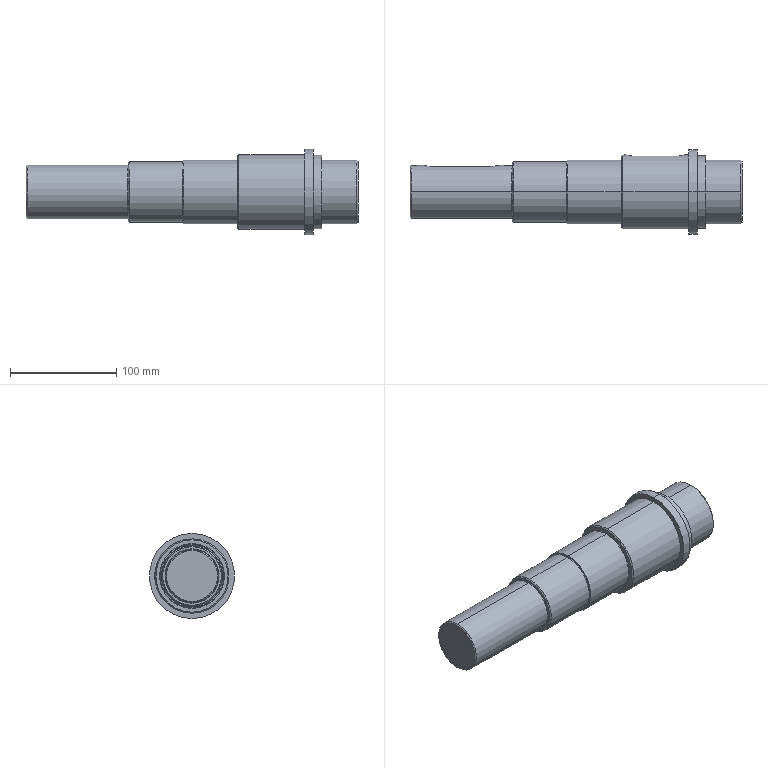Part | SolidWorks | features Chamfer 4, Fillet 2, ICE 2, Revolution 1 | 1 solid | 46 faces | box 312 x 80 x 80 mm | volume 861601 mm3 | cylinder 18 | plane 14 | cone 8 | torus 6 | commonest cylinder face diameters 60 x4 14 x2 20 x2 50 x2 57 x2 69 x2
STEP:
#1=CARTESIAN_POINT('',(199.,0.,30.5));
#2=VERTEX_POINT('',#1);
#3=CARTESIAN_POINT('',(199.,0.,-30.5));
#4=VERTEX_POINT('',#3);
#5=CARTESIAN_POINT('',(199.,0.,0.));
#6=DIRECTION('',(1.,0.,0.));
#7=DIRECTION('',(0.,0.,-1.));
#8=AXIS2_PLACEMENT_3D('',#5,#6,#7);
#9=CIRCLE('',#8,30.5);
#10=EDGE_CURVE('',#2,#4,#9,.T.);
#11=ORIENTED_EDGE('',*,*,#10,.F.);
#12=CARTESIAN_POINT('',(198.5,0.,30.));
#13=VERTEX_POINT('',#12);
#14=CARTESIAN_POINT('',(198.5,0.,30.5));
#15=DIRECTION('',(0.,1.,0.));
#16=DIRECTION('',(0.,0.,1.));
#17=AXIS2_PLACEMENT_3D('',#14,#15,#16);
#18=CIRCLE('',#17,0.5);
#19=EDGE_CURVE('',#2,#13,#18,.T.);
#20=ORIENTED_EDGE('',*,*,#19,.T.);
#21=CARTESIAN_POINT('',(198.5,0.,-30.));
#22=VERTEX_POINT('',#21);
#23=CARTESIAN_POINT('',(198.5,0.,0.));
#24=DIRECTION('',(-1.,0.,0.));
#25=DIRECTION('',(0.,0.,-1.));
#26=AXIS2_PLACEMENT_3D('',#23,#24,#25);
#27=CIRCLE('',#26,30.);
#28=EDGE_CURVE('',#22,#13,#27,.T.);
#29=ORIENTED_EDGE('',*,*,#28,.F.);
#30=CARTESIAN_POINT('',(198.5,0.,-30.5));
#31=DIRECTION('',(0.,-1.,0.));
#32=DIRECTION('',(0.,0.,-1.));
#33=AXIS2_PLACEMENT_3D('',#30,#31,#32);
#34=CIRCLE('',#33,0.5);
#35=EDGE_CURVE('',#4,#22,#34,.T.);
#36=ORIENTED_EDGE('',*,*,#35,.F.);
#37=EDGE_LOOP('',(#11,#20,#29,#36));
#38=FACE_OUTER_BOUND('',#37,.T.);
#39=CARTESIAN_POINT('',(198.5,0.,0.));
#40=DIRECTION('',(1.,0.,0.));
#41=DIRECTION('',(0.,0.,-1.));
#42=AXIS2_PLACEMENT_3D('',#39,#40,#41);
#43=TOROIDAL_SURFACE('',#42,30.5,0.5);
#44=ADVANCED_FACE('',(#38),#43,.F.);
#45=CARTESIAN_POINT('',(96.,0.,27.5));
#46=VERTEX_POINT('',#45);
#47=CARTESIAN_POINT('',(96.,0.,-27.5));
#48=VERTEX_POINT('',#47);
#49=CARTESIAN_POINT('',(96.,0.,0.));
#50=DIRECTION('',(-1.,0.,0.));
#51=DIRECTION('',(0.,0.,-1.));
#52=AXIS2_PLACEMENT_3D('',#49,#50,#51);
#53=CIRCLE('',#52,27.5);
#54=EDGE_CURVE('',#46,#48,#53,.T.);
#55=ORIENTED_EDGE('',*,*,#54,.F.);
#56=CARTESIAN_POINT('',(97.,0.,28.5));
#57=VERTEX_POINT('',#56);
#58=CARTESIAN_POINT('',(96.,0.,27.5));
#59=DIRECTION('',(0.7071,0.,0.7071));
#60=VECTOR('',#59,1000.);
#61=LINE('',#58,#60);
#62=EDGE_CURVE('',#46,#57,#61,.T.);
#63=ORIENTED_EDGE('',*,*,#62,.T.);
#64=CARTESIAN_POINT('',(97.,0.,-28.5));
#65=VERTEX_POINT('',#64);
#66=CARTESIAN_POINT('',(97.,0.,0.));
#67=DIRECTION('',(1.,0.,0.));
#68=DIRECTION('',(0.,0.,-1.));
#69=AXIS2_PLACEMENT_3D('',#66,#67,#68);
#70=CIRCLE('',#69,28.5);
#71=EDGE_CURVE('',#65,#57,#70,.T.);
#72=ORIENTED_EDGE('',*,*,#71,.F.);
#73=CARTESIAN_POINT('',(96.,0.,-27.5));
#74=DIRECTION('',(0.7071,0.,-0.7071));
#75=VECTOR('',#74,1000.);
#76=LINE('',#73,#75);
#77=EDGE_CURVE('',#48,#65,#76,.T.);
#78=ORIENTED_EDGE('',*,*,#77,.F.);
#79=EDGE_LOOP('',(#55,#63,#72,#78));
#80=FACE_OUTER_BOUND('',#79,.T.);
#81=CARTESIAN_POINT('',(96.,0.,0.));
#82=DIRECTION('',(1.,0.,0.));
#83=DIRECTION('',(0.,0.,-1.));
#84=AXIS2_PLACEMENT_3D('',#81,#82,#83);
#85=CONICAL_SURFACE('',#84,27.5,0.7854);
#86=ADVANCED_FACE('',(#80),#85,.T.);
#87=CARTESIAN_POINT('',(199.,0.,34.));
#88=VERTEX_POINT('',#87);
#89=CARTESIAN_POINT('',(199.,0.,-34.));
#90=VERTEX_POINT('',#89);
#91=CARTESIAN_POINT('',(199.,0.,0.));
#92=DIRECTION('',(-1.,0.,0.));
#93=DIRECTION('',(0.,0.,-1.));
#94=AXIS2_PLACEMENT_3D('',#91,#92,#93);
#95=CIRCLE('',#94,34.);
#96=EDGE_CURVE('',#88,#90,#95,.T.);
#97=ORIENTED_EDGE('',*,*,#96,.F.);
#98=CARTESIAN_POINT('',(200.,0.,35.));
#99=VERTEX_POINT('',#98);
#100=CARTESIAN_POINT('',(199.,0.,34.));
#101=DIRECTION('',(0.7071,0.,0.7071));
#102=VECTOR('',#101,1000.);
#103=LINE('',#100,#102);
#104=EDGE_CURVE('',#88,#99,#103,.T.);
#105=ORIENTED_EDGE('',*,*,#104,.T.);
#106=CARTESIAN_POINT('',(200.,0.,-35.));
#107=VERTEX_POINT('',#106);
#108=CARTESIAN_POINT('',(200.,0.,0.));
#109=DIRECTION('',(1.,0.,0.));
#110=DIRECTION('',(0.,0.,-1.));
#111=AXIS2_PLACEMENT_3D('',#108,#109,#110);
#112=CIRCLE('',#111,35.);
#113=EDGE_CURVE('',#107,#99,#112,.T.);
#114=ORIENTED_EDGE('',*,*,#113,.F.);
#115=CARTESIAN_POINT('',(199.,0.,-34.));
#116=DIRECTION('',(0.7071,0.,-0.7071));
#117=VECTOR('',#116,1000.);
#118=LINE('',#115,#117);
#119=EDGE_CURVE('',#90,#107,#118,.T.);
#120=ORIENTED_EDGE('',*,*,#119,.F.);
#121=EDGE_LOOP('',(#97,#105,#114,#120));
#122=FACE_OUTER_BOUND('',#121,.T.);
#123=CARTESIAN_POINT('',(199.,0.,0.));
#124=DIRECTION('',(1.,0.,0.));
#125=DIRECTION('',(0.,0.,-1.));
#126=AXIS2_PLACEMENT_3D('',#123,#124,#125);
#127=CONICAL_SURFACE('',#126,34.,0.7854);
#128=ADVANCED_FACE('',(#122),#127,.T.);
#129=CARTESIAN_POINT('',(96.,0.,25.5));
#130=VERTEX_POINT('',#129);
#131=CARTESIAN_POINT('',(96.,0.,-25.5));
#132=VERTEX_POINT('',#131);
#133=CARTESIAN_POINT('',(96.,0.,0.));
#134=DIRECTION('',(1.,0.,0.));
#135=DIRECTION('',(0.,0.,-1.));
#136=AXIS2_PLACEMENT_3D('',#133,#134,#135);
#137=CIRCLE('',#136,25.5);
#138=EDGE_CURVE('',#130,#132,#137,.T.);
#139=ORIENTED_EDGE('',*,*,#138,.F.);
#140=CARTESIAN_POINT('',(95.5,0.,25.));
#141=VERTEX_POINT('',#140);
#142=CARTESIAN_POINT('',(95.5,0.,25.5));
#143=DIRECTION('',(0.,1.,0.));
#144=DIRECTION('',(0.,0.,1.));
#145=AXIS2_PLACEMENT_3D('',#142,#143,#144);
#146=CIRCLE('',#145,0.5);
#147=EDGE_CURVE('',#130,#141,#146,.T.);
#148=ORIENTED_EDGE('',*,*,#147,.T.);
#149=CARTESIAN_POINT('',(95.5,0.,-25.));
#150=VERTEX_POINT('',#149);
#151=CARTESIAN_POINT('',(95.5,0.,0.));
#152=DIRECTION('',(-1.,0.,0.));
#153=DIRECTION('',(0.,0.,-1.));
#154=AXIS2_PLACEMENT_3D('',#151,#152,#153);
#155=CIRCLE('',#154,25.);
#156=EDGE_CURVE('',#150,#141,#155,.T.);
#157=ORIENTED_EDGE('',*,*,#156,.F.);
#158=CARTESIAN_POINT('',(95.5,0.,-25.5));
#159=DIRECTION('',(0.,-1.,0.));
#160=DIRECTION('',(0.,0.,-1.));
#161=AXIS2_PLACEMENT_3D('',#158,#159,#160);
#162=CIRCLE('',#161,0.5);
#163=EDGE_CURVE('',#132,#150,#162,.T.);
#164=ORIENTED_EDGE('',*,*,#163,.F.);
#165=EDGE_LOOP('',(#139,#148,#157,#164));
#166=FACE_OUTER_BOUND('',#165,.T.);
#167=CARTESIAN_POINT('',(95.5,0.,0.));
#168=DIRECTION('',(1.,0.,0.));
#169=DIRECTION('',(0.,0.,-1.));
#170=AXIS2_PLACEMENT_3D('',#167,#168,#169);
#171=TOROIDAL_SURFACE('',#170,25.5,0.5);
#172=ADVANCED_FACE('',(#166),#171,.F.);
#173=CARTESIAN_POINT('',(148.,0.,29.));
#174=VERTEX_POINT('',#173);
#175=CARTESIAN_POINT('',(148.,0.,-29.));
#176=VERTEX_POINT('',#175);
#177=CARTESIAN_POINT('',(148.,0.,0.));
#178=DIRECTION('',(1.,0.,0.));
#179=DIRECTION('',(0.,0.,-1.));
#180=AXIS2_PLACEMENT_3D('',#177,#178,#179);
#181=CIRCLE('',#180,29.);
#182=EDGE_CURVE('',#174,#176,#181,.T.);
#183=ORIENTED_EDGE('',*,*,#182,.F.);
#184=CARTESIAN_POINT('',(147.5,0.,28.5));
#185=VERTEX_POINT('',#184);
#186=CARTESIAN_POINT('',(147.5,0.,29.));
#187=DIRECTION('',(0.,1.,0.));
#188=DIRECTION('',(0.,0.,1.));
#189=AXIS2_PLACEMENT_3D('',#186,#187,#188);
#190=CIRCLE('',#189,0.5);
#191=EDGE_CURVE('',#174,#185,#190,.T.);
#192=ORIENTED_EDGE('',*,*,#191,.T.);
#193=CARTESIAN_POINT('',(147.5,0.,-28.5));
#194=VERTEX_POINT('',#193);
#195=CARTESIAN_POINT('',(147.5,0.,0.));
#196=DIRECTION('',(-1.,0.,0.));
#197=DIRECTION('',(0.,0.,-1.));
#198=AXIS2_PLACEMENT_3D('',#195,#196,#197);
#199=CIRCLE('',#198,28.5);
#200=EDGE_CURVE('',#194,#185,#199,.T.);
#201=ORIENTED_EDGE('',*,*,#200,.F.);
#202=CARTESIAN_POINT('',(147.5,0.,-29.));
#203=DIRECTION('',(0.,-1.,0.));
#204=DIRECTION('',(0.,0.,-1.));
#205=AXIS2_PLACEMENT_3D('',#202,#203,#204);
#206=CIRCLE('',#205,0.5);
#207=EDGE_CURVE('',#176,#194,#206,.T.);
#208=ORIENTED_EDGE('',*,*,#207,.F.);
#209=EDGE_LOOP('',(#183,#192,#201,#208));
#210=FACE_OUTER_BOUND('',#209,.T.);
#211=CARTESIAN_POINT('',(147.5,0.,0.));
#212=DIRECTION('',(1.,0.,0.));
#213=DIRECTION('',(0.,0.,-1.));
#214=AXIS2_PLACEMENT_3D('',#211,#212,#213);
#215=TOROIDAL_SURFACE('',#214,29.,0.5);
#216=ADVANCED_FACE('',(#210),#215,.F.);
#217=CARTESIAN_POINT('',(312.,0.,-29.));
#218=VERTEX_POINT('',#217);
#219=CARTESIAN_POINT('',(312.,0.,29.));
#220=VERTEX_POINT('',#219);
#221=CARTESIAN_POINT('',(312.,0.,0.));
#222=DIRECTION('',(1.,0.,0.));
#223=DIRECTION('',(0.,0.,1.));
#224=AXIS2_PLACEMENT_3D('',#221,#222,#223);
#225=CIRCLE('',#224,29.);
#226=EDGE_CURVE('',#218,#220,#225,.T.);
#227=ORIENTED_EDGE('',*,*,#226,.F.);
#228=CARTESIAN_POINT('',(311.,0.,-30.));
#229=VERTEX_POINT('',#228);
#230=CARTESIAN_POINT('',(311.,0.,-30.));
#231=DIRECTION('',(-0.7071,0.,-0.7071));
#232=VECTOR('',#231,1000.);
#233=LINE('',#230,#232);
#234=EDGE_CURVE('',#218,#229,#233,.T.);
#235=ORIENTED_EDGE('',*,*,#234,.T.);
#236=CARTESIAN_POINT('',(311.,0.,30.));
#237=VERTEX_POINT('',#236);
#238=CARTESIAN_POINT('',(311.,0.,0.));
#239=DIRECTION('',(-1.,0.,0.));
#240=DIRECTION('',(0.,0.,1.));
#241=AXIS2_PLACEMENT_3D('',#238,#239,#240);
#242=CIRCLE('',#241,30.);
#243=EDGE_CURVE('',#237,#229,#242,.T.);
#244=ORIENTED_EDGE('',*,*,#243,.F.);
#245=CARTESIAN_POINT('',(311.,0.,30.));
#246=DIRECTION('',(-0.7071,0.,0.7071));
#247=VECTOR('',#246,1000.);
#248=LINE('',#245,#247);
#249=EDGE_CURVE('',#220,#237,#248,.T.);
#250=ORIENTED_EDGE('',*,*,#249,.F.);
#251=EDGE_LOOP('',(#227,#235,#244,#250));
#252=FACE_OUTER_BOUND('',#251,.T.);
#253=CARTESIAN_POINT('',(311.,0.,0.));
#254=DIRECTION('',(-1.,0.,0.));
#255=DIRECTION('',(0.,0.,1.));
#256=AXIS2_PLACEMENT_3D('',#253,#254,#255);
#257=CONICAL_SURFACE('',#256,30.,0.7854);
#258=ADVANCED_FACE('',(#252),#257,.T.);
#259=CARTESIAN_POINT('',(0.,0.,24.));
#260=VERTEX_POINT('',#259);
#261=CARTESIAN_POINT('',(0.,0.,-24.));
#262=VERTEX_POINT('',#261);
#263=CARTESIAN_POINT('',(0.,0.,0.));
#264=DIRECTION('',(-1.,0.,0.));
#265=DIRECTION('',(0.,0.,-1.));
#266=AXIS2_PLACEMENT_3D('',#263,#264,#265);
#267=CIRCLE('',#266,24.);
#268=EDGE_CURVE('',#260,#262,#267,.T.);
#269=ORIENTED_EDGE('',*,*,#268,.F.);
#270=CARTESIAN_POINT('',(1.,0.,25.));
#271=VERTEX_POINT('',#270);
#272=CARTESIAN_POINT('',(0.,0.,24.));
#273=DIRECTION('',(0.7071,0.,0.7071));
#274=VECTOR('',#273,1000.);
#275=LINE('',#272,#274);
#276=EDGE_CURVE('',#260,#271,#275,.T.);
#277=ORIENTED_EDGE('',*,*,#276,.T.);
#278=CARTESIAN_POINT('',(1.,0.,-25.));
#279=VERTEX_POINT('',#278);
#280=CARTESIAN_POINT('',(1.,0.,0.));
#281=DIRECTION('',(1.,0.,0.));
#282=DIRECTION('',(0.,0.,-1.));
#283=AXIS2_PLACEMENT_3D('',#280,#281,#282);
#284=CIRCLE('',#283,25.);
#285=EDGE_CURVE('',#279,#271,#284,.T.);
#286=ORIENTED_EDGE('',*,*,#285,.F.);
#287=CARTESIAN_POINT('',(0.,0.,-24.));
#288=DIRECTION('',(0.7071,0.,-0.7071));
#289=VECTOR('',#288,1000.);
#290=LINE('',#287,#289);
#291=EDGE_CURVE('',#262,#279,#290,.T.);
#292=ORIENTED_EDGE('',*,*,#291,.F.);
#293=EDGE_LOOP('',(#269,#277,#286,#292));
#294=FACE_OUTER_BOUND('',#293,.T.);
#295=CARTESIAN_POINT('',(0.,0.,0.));
#296=DIRECTION('',(1.,0.,0.));
#297=DIRECTION('',(0.,0.,-1.));
#298=AXIS2_PLACEMENT_3D('',#295,#296,#297);
#299=CONICAL_SURFACE('',#298,24.,0.7854);
#300=ADVANCED_FACE('',(#294),#299,.T.);
#301=ORIENTED_EDGE('',*,*,#243,.T.);
#302=CARTESIAN_POINT('',(278.,0.,-30.));
#303=VERTEX_POINT('',#302);
#304=CARTESIAN_POINT('',(0.,0.,-30.));
#305=DIRECTION('',(-1.,0.,0.));
#306=VECTOR('',#305,1000.);
#307=LINE('',#304,#306);
#308=EDGE_CURVE('',#229,#303,#307,.T.);
#309=ORIENTED_EDGE('',*,*,#308,.T.);
#310=CARTESIAN_POINT('',(278.,0.,30.));
#311=VERTEX_POINT('',#310);
#312=CARTESIAN_POINT('',(278.,0.,0.));
#313=DIRECTION('',(-1.,0.,0.));
#314=DIRECTION('',(0.,0.,1.));
#315=AXIS2_PLACEMENT_3D('',#312,#313,#314);
#316=CIRCLE('',#315,30.);
#317=EDGE_CURVE('',#311,#303,#316,.T.);
#318=ORIENTED_EDGE('',*,*,#317,.F.);
#319=CARTESIAN_POINT('',(0.,0.,30.));
#320=DIRECTION('',(-1.,0.,0.));
#321=VECTOR('',#320,1000.);
#322=LINE('',#319,#321);
#323=EDGE_CURVE('',#237,#311,#322,.T.);
#324=ORIENTED_EDGE('',*,*,#323,.F.);
#325=EDGE_LOOP('',(#301,#309,#318,#324));
#326=FACE_OUTER_BOUND('',#325,.T.);
#327=CARTESIAN_POINT('',(0.,0.,0.));
#328=DIRECTION('',(-1.,0.,0.));
#329=DIRECTION('',(0.,0.,1.));
#330=AXIS2_PLACEMENT_3D('',#327,#328,#329);
#331=CYLINDRICAL_SURFACE('',#330,30.);
#332=ADVANCED_FACE('',(#326),#331,.T.);
#333=CARTESIAN_POINT('',(278.,0.,34.5));
#334=VERTEX_POINT('',#333);
#335=CARTESIAN_POINT('',(278.,0.,-34.5));
#336=VERTEX_POINT('',#335);
#337=CARTESIAN_POINT('',(278.,0.,0.));
#338=DIRECTION('',(-1.,0.,0.));
#339=DIRECTION('',(0.,0.,1.));
#340=AXIS2_PLACEMENT_3D('',#337,#338,#339);
#341=CIRCLE('',#340,34.5);
#342=EDGE_CURVE('',#334,#336,#341,.T.);
#343=ORIENTED_EDGE('',*,*,#342,.T.);
#344=CARTESIAN_POINT('',(270.,0.,-34.5));
#345=VERTEX_POINT('',#344);
#346=CARTESIAN_POINT('',(0.,0.,-34.5));
#347=DIRECTION('',(-1.,0.,0.));
#348=VECTOR('',#347,1000.);
#349=LINE('',#346,#348);
#350=EDGE_CURVE('',#336,#345,#349,.T.);
#351=ORIENTED_EDGE('',*,*,#350,.T.);
#352=CARTESIAN_POINT('',(270.,0.,34.5));
#353=VERTEX_POINT('',#352);
#354=CARTESIAN_POINT('',(270.,0.,0.));
#355=DIRECTION('',(-1.,0.,0.));
#356=DIRECTION('',(0.,0.,1.));
#357=AXIS2_PLACEMENT_3D('',#354,#355,#356);
#358=CIRCLE('',#357,34.5);
#359=EDGE_CURVE('',#353,#345,#358,.T.);
#360=ORIENTED_EDGE('',*,*,#359,.F.);
#361=CARTESIAN_POINT('',(0.,0.,34.5));
#362=DIRECTION('',(-1.,0.,0.));
#363=VECTOR('',#362,1000.);
#364=LINE('',#361,#363);
#365=EDGE_CURVE('',#334,#353,#364,.T.);
#366=ORIENTED_EDGE('',*,*,#365,.F.);
#367=EDGE_LOOP('',(#343,#351,#360,#366));
#368=FACE_OUTER_BOUND('',#367,.T.);
#369=CARTESIAN_POINT('',(0.,0.,0.));
#370=DIRECTION('',(-1.,0.,0.));
#371=DIRECTION('',(0.,0.,1.));
#372=AXIS2_PLACEMENT_3D('',#369,#370,#371);
#373=CYLINDRICAL_SURFACE('',#372,34.5);
#374=ADVANCED_FACE('',(#368),#373,.T.);
#375=CARTESIAN_POINT('',(270.,0.,40.));
#376=VERTEX_POINT('',#375);
#377=CARTESIAN_POINT('',(270.,0.,-40.));
#378=VERTEX_POINT('',#377);
#379=CARTESIAN_POINT('',(270.,0.,0.));
#380=DIRECTION('',(-1.,0.,0.));
#381=DIRECTION('',(0.,0.,1.));
#382=AXIS2_PLACEMENT_3D('',#379,#380,#381);
#383=CIRCLE('',#382,40.);
#384=EDGE_CURVE('',#376,#378,#383,.T.);
#385=ORIENTED_EDGE('',*,*,#384,.T.);
#386=CARTESIAN_POINT('',(262.,0.,-40.));
#387=VERTEX_POINT('',#386);
#388=CARTESIAN_POINT('',(0.,0.,-40.));
#389=DIRECTION('',(-1.,0.,0.));
#390=VECTOR('',#389,1000.);
#391=LINE('',#388,#390);
#392=EDGE_CURVE('',#378,#387,#391,.T.);
#393=ORIENTED_EDGE('',*,*,#392,.T.);
#394=CARTESIAN_POINT('',(262.,0.,40.));
#395=VERTEX_POINT('',#394);
#396=CARTESIAN_POINT('',(262.,0.,0.));
#397=DIRECTION('',(-1.,0.,0.));
#398=DIRECTION('',(0.,0.,1.));
#399=AXIS2_PLACEMENT_3D('',#396,#397,#398);
#400=CIRCLE('',#399,40.);
#401=EDGE_CURVE('',#395,#387,#400,.T.);
#402=ORIENTED_EDGE('',*,*,#401,.F.);
#403=CARTESIAN_POINT('',(0.,0.,40.));
#404=DIRECTION('',(-1.,0.,0.));
#405=VECTOR('',#404,1000.);
#406=LINE('',#403,#405);
#407=EDGE_CURVE('',#376,#395,#406,.T.);
#408=ORIENTED_EDGE('',*,*,#407,.F.);
#409=EDGE_LOOP('',(#385,#393,#402,#408));
#410=FACE_OUTER_BOUND('',#409,.T.);
#411=CARTESIAN_POINT('',(0.,0.,0.));
#412=DIRECTION('',(-1.,0.,0.));
#413=DIRECTION('',(0.,0.,1.));
#414=AXIS2_PLACEMENT_3D('',#411,#412,#413);
#415=CYLINDRICAL_SURFACE('',#414,40.);
#416=ADVANCED_FACE('',(#410),#415,.T.);
#417=CARTESIAN_POINT('',(198.5,0.,0.));
#418=DIRECTION('',(-1.,0.,0.));
#419=DIRECTION('',(0.,0.,-1.));
#420=AXIS2_PLACEMENT_3D('',#417,#418,#419);
#421=CIRCLE('',#420,30.);
#422=EDGE_CURVE('',#13,#22,#421,.T.);
#423=ORIENTED_EDGE('',*,*,#422,.T.);
#424=CARTESIAN_POINT('',(148.,0.,-30.));
#425=VERTEX_POINT('',#424);
#426=CARTESIAN_POINT('',(0.,0.,-30.));
#427=DIRECTION('',(-1.,0.,0.));
#428=VECTOR('',#427,1000.);
#429=LINE('',#426,#428);
#430=EDGE_CURVE('',#22,#425,#429,.T.);
#431=ORIENTED_EDGE('',*,*,#430,.T.);
#432=CARTESIAN_POINT('',(148.,0.,30.));
#433=VERTEX_POINT('',#432);
#434=CARTESIAN_POINT('',(148.,0.,0.));
#435=DIRECTION('',(-1.,0.,0.));
#436=DIRECTION('',(0.,0.,1.));
#437=AXIS2_PLACEMENT_3D('',#434,#435,#436);
#438=CIRCLE('',#437,30.);
#439=EDGE_CURVE('',#433,#425,#438,.T.);
#440=ORIENTED_EDGE('',*,*,#439,.F.);
#441=CARTESIAN_POINT('',(0.,0.,30.));
#442=DIRECTION('',(-1.,0.,0.));
#443=VECTOR('',#442,1000.);
#444=LINE('',#441,#443);
#445=EDGE_CURVE('',#13,#433,#444,.T.);
#446=ORIENTED_EDGE('',*,*,#445,.F.);
#447=EDGE_LOOP('',(#423,#431,#440,#446));
#448=FACE_OUTER_BOUND('',#447,.T.);
#449=CARTESIAN_POINT('',(0.,0.,0.));
#450=DIRECTION('',(-1.,0.,0.));
#451=DIRECTION('',(0.,0.,1.));
#452=AXIS2_PLACEMENT_3D('',#449,#450,#451);
#453=CYLINDRICAL_SURFACE('',#452,30.);
#454=ADVANCED_FACE('',(#448),#453,.T.);
#455=CARTESIAN_POINT('',(147.5,0.,0.));
#456=DIRECTION('',(-1.,0.,0.));
#457=DIRECTION('',(0.,0.,-1.));
#458=AXIS2_PLACEMENT_3D('',#455,#456,#457);
#459=CIRCLE('',#458,28.5);
#460=EDGE_CURVE('',#185,#194,#459,.T.);
#461=ORIENTED_EDGE('',*,*,#460,.T.);
#462=CARTESIAN_POINT('',(0.,0.,-28.5));
#463=DIRECTION('',(-1.,0.,0.));
#464=VECTOR('',#463,1000.);
#465=LINE('',#462,#464);
#466=EDGE_CURVE('',#194,#65,#465,.T.);
#467=ORIENTED_EDGE('',*,*,#466,.T.);
#468=ORIENTED_EDGE('',*,*,#71,.T.);
#469=CARTESIAN_POINT('',(0.,0.,28.5));
#470=DIRECTION('',(-1.,0.,0.));
#471=VECTOR('',#470,1000.);
#472=LINE('',#469,#471);
#473=EDGE_CURVE('',#185,#57,#472,.T.);
#474=ORIENTED_EDGE('',*,*,#473,.F.);
#475=EDGE_LOOP('',(#461,#467,#468,#474));
#476=FACE_OUTER_BOUND('',#475,.T.);
#477=CARTESIAN_POINT('',(0.,0.,0.));
#478=DIRECTION('',(-1.,0.,0.));
#479=DIRECTION('',(0.,0.,1.));
#480=AXIS2_PLACEMENT_3D('',#477,#478,#479);
#481=CYLINDRICAL_SURFACE('',#480,28.5);
#482=ADVANCED_FACE('',(#476),#481,.T.);
#483=CARTESIAN_POINT('',(20.,24.,-7.));
#484=VERTEX_POINT('',#483);
#485=CARTESIAN_POINT('',(20.,24.,7.));
#486=VERTEX_POINT('',#485);
#487=CARTESIAN_POINT('',(20.,24.,-7.));
#488=CARTESIAN_POINT('',(19.535,24.,-7.));
#489=CARTESIAN_POINT('',(19.079,24.014,-6.954));
#490=CARTESIAN_POINT('',(18.405,24.052,-6.82));
#491=CARTESIAN_POINT('',(18.183,24.068,-6.764));
#492=CARTESIAN_POINT('',(17.742,24.105,-6.63));
#493=CARTESIAN_POINT('',(17.524,24.126,-6.551));
#494=CARTESIAN_POINT('',(16.889,24.197,-6.287));
#495=CARTESIAN_POINT('',(16.488,24.253,-6.072));
#496=CARTESIAN_POINT('',(15.919,24.344,-5.692));
#497=CARTESIAN_POINT('',(15.733,24.376,-5.554));
#498=CARTESIAN_POINT('',(15.38,24.44,-5.263));
#499=CARTESIAN_POINT('',(15.211,24.473,-5.11));
#500=CARTESIAN_POINT('',(14.729,24.57,-4.629));
#501=CARTESIAN_POINT('',(14.44,24.634,-4.278));
#502=CARTESIAN_POINT('',(13.929,24.755,-3.514));
#503=CARTESIAN_POINT('',(13.713,24.809,-3.11));
#504=CARTESIAN_POINT('',(13.45,24.878,-2.48));
#505=CARTESIAN_POINT('',(13.373,24.898,-2.265));
#506=CARTESIAN_POINT('',(13.238,24.934,-1.825));
#507=CARTESIAN_POINT('',(13.181,24.95,-1.6));
#508=CARTESIAN_POINT('',(13.046,24.987,-0.9213));
#509=CARTESIAN_POINT('',(13.,25.,-0.4657));
#510=CARTESIAN_POINT('',(13.,25.,0.4524));
#511=CARTESIAN_POINT('',(13.045,24.987,0.9188));
#512=CARTESIAN_POINT('',(13.225,24.938,1.818));
#513=CARTESIAN_POINT('',(13.358,24.902,2.256));
#514=CARTESIAN_POINT('',(13.622,24.833,2.894));
#515=CARTESIAN_POINT('',(13.721,24.808,3.103));
#516=CARTESIAN_POINT('',(13.937,24.754,3.506));
#517=CARTESIAN_POINT('',(14.054,24.725,3.701));
#518=CARTESIAN_POINT('',(14.307,24.666,4.079));
#519=CARTESIAN_POINT('',(14.442,24.635,4.262));
#520=CARTESIAN_POINT('',(14.732,24.571,4.615));
#521=CARTESIAN_POINT('',(14.887,24.538,4.786));
#522=CARTESIAN_POINT('',(15.372,24.44,5.272));
#523=CARTESIAN_POINT('',(15.722,24.375,5.56));
#524=CARTESIAN_POINT('',(16.478,24.254,6.067));
#525=CARTESIAN_POINT('',(16.888,24.197,6.287));
#526=CARTESIAN_POINT('',(17.731,24.103,6.638));
#527=CARTESIAN_POINT('',(18.168,24.066,6.772));
#528=CARTESIAN_POINT('',(18.844,24.027,6.908));
#529=CARTESIAN_POINT('',(19.075,24.017,6.942));
#530=CARTESIAN_POINT('',(19.536,24.003,6.988));
#531=CARTESIAN_POINT('',(19.768,24.,7.));
#532=CARTESIAN_POINT('',(20.,24.,7.));
#533=B_SPLINE_CURVE_WITH_KNOTS('',3,(#487,#488,#489,#490,#491,#492,#493,#494,#495,#496,#497,#498,#499,#500,#501,#502,#503,#504,#505,#506,#507,#508,#509,#510,#511,#512,#513,#514,#515,#516,#517,#518,#519,#520,#521,#522,#523,#524,#525,#526,#527,#528,#529,#530,#531,#532),.UNSPECIFIED.,.F.,.F.,(4,2,2,2,2,2,2,2,2,2,2,2,2,2,2,2,2,2,2,2,2,2,4),(0.,0.001374,0.002061,0.002749,0.004123,0.00481,0.005497,0.006871,0.008246,0.008933,0.00962,0.01099,0.01237,0.01374,0.01443,0.01512,0.0158,0.01649,0.01787,0.01924,0.02061,0.0213,0.02199),.UNSPECIFIED.);
#534=EDGE_CURVE('',#484,#486,#533,.T.);
#535=ORIENTED_EDGE('',*,*,#534,.F.);
#536=CARTESIAN_POINT('',(76.,24.,-7.));
#537=VERTEX_POINT('',#536);
#538=CARTESIAN_POINT('',(0.,24.,-7.));
#539=DIRECTION('',(-1.,0.,0.));
#540=VECTOR('',#539,1000.);
#541=LINE('',#538,#540);
#542=EDGE_CURVE('',#537,#484,#541,.T.);
#543=ORIENTED_EDGE('',*,*,#542,.F.);
#544=CARTESIAN_POINT('',(76.,24.,7.));
#545=VERTEX_POINT('',#544);
#546=CARTESIAN_POINT('',(76.,24.,7.));
#547=CARTESIAN_POINT('',(76.465,24.,7.));
#548=CARTESIAN_POINT('',(76.921,24.014,6.954));
#549=CARTESIAN_POINT('',(77.595,24.052,6.82));
#550=CARTESIAN_POINT('',(77.817,24.068,6.764));
#551=CARTESIAN_POINT('',(78.258,24.105,6.63));
#552=CARTESIAN_POINT('',(78.476,24.126,6.551));
#553=CARTESIAN_POINT('',(79.111,24.197,6.287));
#554=CARTESIAN_POINT('',(79.512,24.253,6.072));
#555=CARTESIAN_POINT('',(80.081,24.344,5.692));
#556=CARTESIAN_POINT('',(80.267,24.376,5.554));
#557=CARTESIAN_POINT('',(80.62,24.44,5.263));
#558=CARTESIAN_POINT('',(80.789,24.473,5.11));
#559=CARTESIAN_POINT('',(81.271,24.57,4.629));
#560=CARTESIAN_POINT('',(81.56,24.634,4.278));
#561=CARTESIAN_POINT('',(82.071,24.755,3.514));
#562=CARTESIAN_POINT('',(82.287,24.809,3.11));
#563=CARTESIAN_POINT('',(82.55,24.878,2.48));
#564=CARTESIAN_POINT('',(82.627,24.898,2.265));
#565=CARTESIAN_POINT('',(82.762,24.934,1.825));
#566=CARTESIAN_POINT('',(82.819,24.95,1.6));
#567=CARTESIAN_POINT('',(82.954,24.987,0.9213));
#568=CARTESIAN_POINT('',(83.,25.,0.4657));
#569=CARTESIAN_POINT('',(83.,25.,-0.4524));
#570=CARTESIAN_POINT('',(82.955,24.987,-0.9188));
#571=CARTESIAN_POINT('',(82.775,24.938,-1.818));
#572=CARTESIAN_POINT('',(82.642,24.902,-2.256));
#573=CARTESIAN_POINT('',(82.378,24.833,-2.894));
#574=CARTESIAN_POINT('',(82.279,24.808,-3.103));
#575=CARTESIAN_POINT('',(82.063,24.754,-3.506));
#576=CARTESIAN_POINT('',(81.946,24.725,-3.701));
#577=CARTESIAN_POINT('',(81.693,24.666,-4.079));
#578=CARTESIAN_POINT('',(81.558,24.635,-4.262));
#579=CARTESIAN_POINT('',(81.268,24.571,-4.615));
#580=CARTESIAN_POINT('',(81.113,24.538,-4.786));
#581=CARTESIAN_POINT('',(80.628,24.44,-5.272));
#582=CARTESIAN_POINT('',(80.278,24.375,-5.56));
#583=CARTESIAN_POINT('',(79.522,24.254,-6.067));
#584=CARTESIAN_POINT('',(79.112,24.197,-6.287));
#585=CARTESIAN_POINT('',(78.269,24.103,-6.638));
#586=CARTESIAN_POINT('',(77.832,24.066,-6.772));
#587=CARTESIAN_POINT('',(77.156,24.027,-6.908));
#588=CARTESIAN_POINT('',(76.925,24.017,-6.942));
#589=CARTESIAN_POINT('',(76.464,24.003,-6.988));
#590=CARTESIAN_POINT('',(76.232,24.,-7.));
#591=CARTESIAN_POINT('',(76.,24.,-7.));
#592=B_SPLINE_CURVE_WITH_KNOTS('',3,(#546,#547,#548,#549,#550,#551,#552,#553,#554,#555,#556,#557,#558,#559,#560,#561,#562,#563,#564,#565,#566,#567,#568,#569,#570,#571,#572,#573,#574,#575,#576,#577,#578,#579,#580,#581,#582,#583,#584,#585,#586,#587,#588,#589,#590,#591),.UNSPECIFIED.,.F.,.F.,(4,2,2,2,2,2,2,2,2,2,2,2,2,2,2,2,2,2,2,2,2,2,4),(0.,0.001374,0.002061,0.002749,0.004123,0.00481,0.005497,0.006871,0.008246,0.008933,0.00962,0.01099,0.01237,0.01374,0.01443,0.01512,0.0158,0.01649,0.01787,0.01924,0.02061,0.0213,0.02199),.UNSPECIFIED.);
#593=EDGE_CURVE('',#545,#537,#592,.T.);
#594=ORIENTED_EDGE('',*,*,#593,.F.);
#595=CARTESIAN_POINT('',(0.,24.,7.));
#596=DIRECTION('',(1.,0.,0.));
#597=VECTOR('',#596,1000.);
#598=LINE('',#595,#597);
#599=EDGE_CURVE('',#486,#545,#598,.T.);
#600=ORIENTED_EDGE('',*,*,#599,.F.);
#601=EDGE_LOOP('',(#535,#543,#594,#600));
#602=FACE_BOUND('',#601,.T.);
#603=CARTESIAN_POINT('',(95.5,0.,0.));
#604=DIRECTION('',(-1.,0.,0.));
#605=DIRECTION('',(0.,0.,-1.));
#606=AXIS2_PLACEMENT_3D('',#603,#604,#605);
#607=CIRCLE('',#606,25.);
#608=EDGE_CURVE('',#141,#150,#607,.T.);
#609=ORIENTED_EDGE('',*,*,#608,.T.);
#610=CARTESIAN_POINT('',(0.,0.,-25.));
#611=DIRECTION('',(-1.,0.,0.));
#612=VECTOR('',#611,1000.);
#613=LINE('',#610,#612);
#614=EDGE_CURVE('',#150,#279,#613,.T.);
#615=ORIENTED_EDGE('',*,*,#614,.T.);
#616=ORIENTED_EDGE('',*,*,#285,.T.);
#617=CARTESIAN_POINT('',(0.,0.,25.));
#618=DIRECTION('',(-1.,0.,0.));
#619=VECTOR('',#618,1000.);
#620=LINE('',#617,#619);
#621=EDGE_CURVE('',#141,#271,#620,.T.);
#622=ORIENTED_EDGE('',*,*,#621,.F.);
#623=EDGE_LOOP('',(#609,#615,#616,#622));
#624=FACE_OUTER_BOUND('',#623,.T.);
#625=CARTESIAN_POINT('',(0.,0.,0.));
#626=DIRECTION('',(-1.,0.,0.));
#627=DIRECTION('',(0.,0.,1.));
#628=AXIS2_PLACEMENT_3D('',#625,#626,#627);
#629=CYLINDRICAL_SURFACE('',#628,25.);
#630=ADVANCED_FACE('',(#602,#624),#629,.T.);
#631=CARTESIAN_POINT('',(212.5,33.541,-10.));
#632=VERTEX_POINT('',#631);
#633=CARTESIAN_POINT('',(212.5,33.541,10.));
#634=VERTEX_POINT('',#633);
#635=CARTESIAN_POINT('',(212.5,33.541,-10.));
#636=CARTESIAN_POINT('',(211.836,33.541,-10.));
#637=CARTESIAN_POINT('',(211.183,33.561,-9.934));
#638=CARTESIAN_POINT('',(210.222,33.617,-9.742));
#639=CARTESIAN_POINT('',(209.904,33.64,-9.663));
#640=CARTESIAN_POINT('',(209.274,33.694,-9.471));
#641=CARTESIAN_POINT('',(208.962,33.726,-9.359));
#642=CARTESIAN_POINT('',(208.055,33.829,-8.982));
#643=CARTESIAN_POINT('',(207.482,33.91,-8.675));
#644=CARTESIAN_POINT('',(206.669,34.043,-8.131));
#645=CARTESIAN_POINT('',(206.405,34.089,-7.934));
#646=CARTESIAN_POINT('',(205.899,34.183,-7.519));
#647=CARTESIAN_POINT('',(205.659,34.231,-7.301));
#648=CARTESIAN_POINT('',(204.971,34.373,-6.613));
#649=CARTESIAN_POINT('',(204.558,34.467,-6.112));
#650=CARTESIAN_POINT('',(203.827,34.642,-5.02));
#651=CARTESIAN_POINT('',(203.518,34.722,-4.444));
#652=CARTESIAN_POINT('',(203.143,34.822,-3.543));
#653=CARTESIAN_POINT('',(203.032,34.852,-3.236));
#654=CARTESIAN_POINT('',(202.841,34.904,-2.608));
#655=CARTESIAN_POINT('',(202.759,34.927,-2.286));
#656=CARTESIAN_POINT('',(202.565,34.981,-1.317));
#657=CARTESIAN_POINT('',(202.501,35.,-0.6655));
#658=CARTESIAN_POINT('',(202.499,35.,0.6464));
#659=CARTESIAN_POINT('',(202.565,34.981,1.313));
#660=CARTESIAN_POINT('',(202.821,34.909,2.598));
#661=CARTESIAN_POINT('',(203.011,34.857,3.223));
#662=CARTESIAN_POINT('',(203.389,34.756,4.135));
#663=CARTESIAN_POINT('',(203.531,34.719,4.433));
#664=CARTESIAN_POINT('',(203.839,34.641,5.009));
#665=CARTESIAN_POINT('',(204.006,34.599,5.288));
#666=CARTESIAN_POINT('',(204.367,34.512,5.828));
#667=CARTESIAN_POINT('',(204.561,34.467,6.089));
#668=CARTESIAN_POINT('',(204.974,34.374,6.593));
#669=CARTESIAN_POINT('',(205.196,34.326,6.838));
#670=CARTESIAN_POINT('',(205.888,34.183,7.531));
#671=CARTESIAN_POINT('',(206.389,34.089,7.942));
#672=CARTESIAN_POINT('',(207.469,33.912,8.666));
#673=CARTESIAN_POINT('',(208.054,33.829,8.981));
#674=CARTESIAN_POINT('',(209.259,33.692,9.483));
#675=CARTESIAN_POINT('',(209.882,33.637,9.674));
#676=CARTESIAN_POINT('',(210.849,33.58,9.868));
#677=CARTESIAN_POINT('',(211.178,33.565,9.918));
#678=CARTESIAN_POINT('',(211.837,33.546,9.983));
#679=CARTESIAN_POINT('',(212.168,33.541,10.));
#680=CARTESIAN_POINT('',(212.5,33.541,10.));
#681=B_SPLINE_CURVE_WITH_KNOTS('',3,(#635,#636,#637,#638,#639,#640,#641,#642,#643,#644,#645,#646,#647,#648,#649,#650,#651,#652,#653,#654,#655,#656,#657,#658,#659,#660,#661,#662,#663,#664,#665,#666,#667,#668,#669,#670,#671,#672,#673,#674,#675,#676,#677,#678,#679,#680),.UNSPECIFIED.,.F.,.F.,(4,2,2,2,2,2,2,2,2,2,2,2,2,2,2,2,2,2,2,2,2,2,4),(0.,0.001964,0.002945,0.003927,0.005891,0.006873,0.007855,0.009818,0.01178,0.01276,0.01375,0.01571,0.01767,0.01964,0.02062,0.0216,0.02258,0.02356,0.02553,0.02749,0.02945,0.03044,0.03142),.UNSPECIFIED.);
#682=EDGE_CURVE('',#632,#634,#681,.T.);
#683=ORIENTED_EDGE('',*,*,#682,.F.);
#684=CARTESIAN_POINT('',(248.5,33.541,-10.));
#685=VERTEX_POINT('',#684);
#686=CARTESIAN_POINT('',(0.,33.541,-10.));
#687=DIRECTION('',(-1.,0.,0.));
#688=VECTOR('',#687,1000.);
#689=LINE('',#686,#688);
#690=EDGE_CURVE('',#685,#632,#689,.T.);
#691=ORIENTED_EDGE('',*,*,#690,.F.);
#692=CARTESIAN_POINT('',(248.5,33.541,10.));
#693=VERTEX_POINT('',#692);
#694=CARTESIAN_POINT('',(248.5,33.541,10.));
#695=CARTESIAN_POINT('',(249.164,33.541,10.));
#696=CARTESIAN_POINT('',(249.817,33.561,9.934));
#697=CARTESIAN_POINT('',(250.778,33.617,9.742));
#698=CARTESIAN_POINT('',(251.096,33.64,9.663));
#699=CARTESIAN_POINT('',(251.726,33.694,9.471));
#700=CARTESIAN_POINT('',(252.038,33.726,9.359));
#701=CARTESIAN_POINT('',(252.945,33.829,8.982));
#702=CARTESIAN_POINT('',(253.518,33.91,8.675));
#703=CARTESIAN_POINT('',(254.331,34.043,8.131));
#704=CARTESIAN_POINT('',(254.595,34.089,7.934));
#705=CARTESIAN_POINT('',(255.101,34.183,7.519));
#706=CARTESIAN_POINT('',(255.341,34.231,7.301));
#707=CARTESIAN_POINT('',(256.029,34.373,6.613));
#708=CARTESIAN_POINT('',(256.442,34.467,6.112));
#709=CARTESIAN_POINT('',(257.173,34.642,5.02));
#710=CARTESIAN_POINT('',(257.482,34.722,4.444));
#711=CARTESIAN_POINT('',(257.857,34.822,3.543));
#712=CARTESIAN_POINT('',(257.968,34.852,3.236));
#713=CARTESIAN_POINT('',(258.159,34.904,2.608));
#714=CARTESIAN_POINT('',(258.241,34.927,2.286));
#715=CARTESIAN_POINT('',(258.435,34.981,1.317));
#716=CARTESIAN_POINT('',(258.499,35.,0.6655));
#717=CARTESIAN_POINT('',(258.501,35.,-0.6464));
#718=CARTESIAN_POINT('',(258.435,34.981,-1.313));
#719=CARTESIAN_POINT('',(258.179,34.909,-2.598));
#720=CARTESIAN_POINT('',(257.989,34.857,-3.223));
#721=CARTESIAN_POINT('',(257.611,34.756,-4.135));
#722=CARTESIAN_POINT('',(257.469,34.719,-4.433));
#723=CARTESIAN_POINT('',(257.161,34.641,-5.009));
#724=CARTESIAN_POINT('',(256.994,34.599,-5.288));
#725=CARTESIAN_POINT('',(256.633,34.512,-5.828));
#726=CARTESIAN_POINT('',(256.439,34.467,-6.089));
#727=CARTESIAN_POINT('',(256.026,34.374,-6.593));
#728=CARTESIAN_POINT('',(255.804,34.326,-6.838));
#729=CARTESIAN_POINT('',(255.112,34.183,-7.531));
#730=CARTESIAN_POINT('',(254.611,34.089,-7.942));
#731=CARTESIAN_POINT('',(253.531,33.912,-8.666));
#732=CARTESIAN_POINT('',(252.946,33.829,-8.981));
#733=CARTESIAN_POINT('',(251.741,33.692,-9.483));
#734=CARTESIAN_POINT('',(251.118,33.637,-9.674));
#735=CARTESIAN_POINT('',(250.151,33.58,-9.868));
#736=CARTESIAN_POINT('',(249.822,33.565,-9.918));
#737=CARTESIAN_POINT('',(249.163,33.546,-9.983));
#738=CARTESIAN_POINT('',(248.832,33.541,-10.));
#739=CARTESIAN_POINT('',(248.5,33.541,-10.));
#740=B_SPLINE_CURVE_WITH_KNOTS('',3,(#694,#695,#696,#697,#698,#699,#700,#701,#702,#703,#704,#705,#706,#707,#708,#709,#710,#711,#712,#713,#714,#715,#716,#717,#718,#719,#720,#721,#722,#723,#724,#725,#726,#727,#728,#729,#730,#731,#732,#733,#734,#735,#736,#737,#738,#739),.UNSPECIFIED.,.F.,.F.,(4,2,2,2,2,2,2,2,2,2,2,2,2,2,2,2,2,2,2,2,2,2,4),(0.,0.001964,0.002945,0.003927,0.005891,0.006873,0.007855,0.009818,0.01178,0.01276,0.01375,0.01571,0.01767,0.01964,0.02062,0.0216,0.02258,0.02356,0.02553,0.02749,0.02945,0.03044,0.03142),.UNSPECIFIED.);
#741=EDGE_CURVE('',#693,#685,#740,.T.);
#742=ORIENTED_EDGE('',*,*,#741,.F.);
#743=CARTESIAN_POINT('',(0.,33.541,10.));
#744=DIRECTION('',(1.,0.,0.));
#745=VECTOR('',#744,1000.);
#746=LINE('',#743,#745);
#747=EDGE_CURVE('',#634,#693,#746,.T.);
#748=ORIENTED_EDGE('',*,*,#747,.F.);
#749=EDGE_LOOP('',(#683,#691,#742,#748));
#750=FACE_BOUND('',#749,.T.);
#751=CARTESIAN_POINT('',(262.,0.,35.));
#752=VERTEX_POINT('',#751);
#753=CARTESIAN_POINT('',(262.,0.,-35.));
#754=VERTEX_POINT('',#753);
#755=CARTESIAN_POINT('',(262.,0.,0.));
#756=DIRECTION('',(-1.,0.,0.));
#757=DIRECTION('',(0.,0.,1.));
#758=AXIS2_PLACEMENT_3D('',#755,#756,#757);
#759=CIRCLE('',#758,35.);
#760=EDGE_CURVE('',#752,#754,#759,.T.);
#761=ORIENTED_EDGE('',*,*,#760,.T.);
#762=CARTESIAN_POINT('',(0.,0.,-35.));
#763=DIRECTION('',(-1.,0.,0.));
#764=VECTOR('',#763,1000.);
#765=LINE('',#762,#764);
#766=EDGE_CURVE('',#754,#107,#765,.T.);
#767=ORIENTED_EDGE('',*,*,#766,.T.);
#768=ORIENTED_EDGE('',*,*,#113,.T.);
#769=CARTESIAN_POINT('',(0.,0.,35.));
#770=DIRECTION('',(-1.,0.,0.));
#771=VECTOR('',#770,1000.);
#772=LINE('',#769,#771);
#773=EDGE_CURVE('',#752,#99,#772,.T.);
#774=ORIENTED_EDGE('',*,*,#773,.F.);
#775=EDGE_LOOP('',(#761,#767,#768,#774));
#776=FACE_OUTER_BOUND('',#775,.T.);
#777=CARTESIAN_POINT('',(0.,0.,0.));
#778=DIRECTION('',(-1.,0.,0.));
#779=DIRECTION('',(0.,0.,1.));
#780=AXIS2_PLACEMENT_3D('',#777,#778,#779);
#781=CYLINDRICAL_SURFACE('',#780,35.);
#782=ADVANCED_FACE('',(#750,#776),#781,.T.);
#783=ORIENTED_EDGE('',*,*,#766,.F.);
#784=CARTESIAN_POINT('',(262.,0.,0.));
#785=DIRECTION('',(-1.,0.,0.));
#786=DIRECTION('',(0.,0.,1.));
#787=AXIS2_PLACEMENT_3D('',#784,#785,#786);
#788=CIRCLE('',#787,35.);
#789=EDGE_CURVE('',#754,#752,#788,.T.);
#790=ORIENTED_EDGE('',*,*,#789,.T.);
#791=ORIENTED_EDGE('',*,*,#773,.T.);
#792=CARTESIAN_POINT('',(200.,0.,0.));
#793=DIRECTION('',(1.,0.,0.));
#794=DIRECTION('',(0.,0.,-1.));
#795=AXIS2_PLACEMENT_3D('',#792,#793,#794);
#796=CIRCLE('',#795,35.);
#797=EDGE_CURVE('',#99,#107,#796,.T.);
#798=ORIENTED_EDGE('',*,*,#797,.T.);
#799=EDGE_LOOP('',(#783,#790,#791,#798));
#800=FACE_OUTER_BOUND('',#799,.T.);
#801=CARTESIAN_POINT('',(0.,0.,0.));
#802=DIRECTION('',(-1.,0.,0.));
#803=DIRECTION('',(0.,0.,1.));
#804=AXIS2_PLACEMENT_3D('',#801,#802,#803);
#805=CYLINDRICAL_SURFACE('',#804,35.);
#806=ADVANCED_FACE('',(#800),#805,.T.);
#807=ORIENTED_EDGE('',*,*,#614,.F.);
#808=ORIENTED_EDGE('',*,*,#156,.T.);
#809=ORIENTED_EDGE('',*,*,#621,.T.);
#810=CARTESIAN_POINT('',(1.,0.,0.));
#811=DIRECTION('',(1.,0.,0.));
#812=DIRECTION('',(0.,0.,-1.));
#813=AXIS2_PLACEMENT_3D('',#810,#811,#812);
#814=CIRCLE('',#813,25.);
#815=EDGE_CURVE('',#271,#279,#814,.T.);
#816=ORIENTED_EDGE('',*,*,#815,.T.);
#817=EDGE_LOOP('',(#807,#808,#809,#816));
#818=FACE_OUTER_BOUND('',#817,.T.);
#819=CARTESIAN_POINT('',(0.,0.,0.));
#820=DIRECTION('',(-1.,0.,0.));
#821=DIRECTION('',(0.,0.,1.));
#822=AXIS2_PLACEMENT_3D('',#819,#820,#821);
#823=CYLINDRICAL_SURFACE('',#822,25.);
#824=ADVANCED_FACE('',(#818),#823,.T.);
#825=CARTESIAN_POINT('',(0.,0.,0.));
#826=DIRECTION('',(-1.,0.,0.));
#827=DIRECTION('',(0.,0.,-1.));
#828=AXIS2_PLACEMENT_3D('',#825,#826,#827);
#829=CIRCLE('',#828,24.);
#830=EDGE_CURVE('',#262,#260,#829,.T.);
#831=ORIENTED_EDGE('',*,*,#830,.T.);
#832=ORIENTED_EDGE('',*,*,#268,.T.);
#833=EDGE_LOOP('',(#831,#832));
#834=FACE_OUTER_BOUND('',#833,.T.);
#835=CARTESIAN_POINT('',(0.,0.,0.));
#836=DIRECTION('',(1.,0.,0.));
#837=DIRECTION('',(0.,0.,-1.));
#838=AXIS2_PLACEMENT_3D('',#835,#836,#837);
#839=PLANE('',#838);
#840=ADVANCED_FACE('',(#834),#839,.F.);
#841=CARTESIAN_POINT('',(96.,0.,0.));
#842=DIRECTION('',(-1.,0.,0.));
#843=DIRECTION('',(0.,0.,-1.));
#844=AXIS2_PLACEMENT_3D('',#841,#842,#843);
#845=CIRCLE('',#844,27.5);
#846=EDGE_CURVE('',#48,#46,#845,.T.);
#847=ORIENTED_EDGE('',*,*,#846,.T.);
#848=ORIENTED_EDGE('',*,*,#54,.T.);
#849=EDGE_LOOP('',(#847,#848));
#850=FACE_OUTER_BOUND('',#849,.T.);
#851=CARTESIAN_POINT('',(96.,0.,0.));
#852=DIRECTION('',(1.,0.,0.));
#853=DIRECTION('',(0.,0.,-1.));
#854=AXIS2_PLACEMENT_3D('',#851,#852,#853);
#855=CIRCLE('',#854,25.5);
#856=EDGE_CURVE('',#132,#130,#855,.T.);
#857=ORIENTED_EDGE('',*,*,#856,.T.);
#858=ORIENTED_EDGE('',*,*,#138,.T.);
#859=EDGE_LOOP('',(#857,#858));
#860=FACE_BOUND('',#859,.T.);
#861=CARTESIAN_POINT('',(96.,25.,0.));
#862=DIRECTION('',(1.,0.,0.));
#863=DIRECTION('',(0.,0.,-1.));
#864=AXIS2_PLACEMENT_3D('',#861,#862,#863);
#865=PLANE('',#864);
#866=ADVANCED_FACE('',(#850,#860),#865,.F.);
#867=ORIENTED_EDGE('',*,*,#466,.F.);
#868=ORIENTED_EDGE('',*,*,#200,.T.);
#869=ORIENTED_EDGE('',*,*,#473,.T.);
#870=CARTESIAN_POINT('',(97.,0.,0.));
#871=DIRECTION('',(1.,0.,0.));
#872=DIRECTION('',(0.,0.,-1.));
#873=AXIS2_PLACEMENT_3D('',#870,#871,#872);
#874=CIRCLE('',#873,28.5);
#875=EDGE_CURVE('',#57,#65,#874,.T.);
#876=ORIENTED_EDGE('',*,*,#875,.T.);
#877=EDGE_LOOP('',(#867,#868,#869,#876));
#878=FACE_OUTER_BOUND('',#877,.T.);
#879=CARTESIAN_POINT('',(0.,0.,0.));
#880=DIRECTION('',(-1.,0.,0.));
#881=DIRECTION('',(0.,0.,1.));
#882=AXIS2_PLACEMENT_3D('',#879,#880,#881);
#883=CYLINDRICAL_SURFACE('',#882,28.5);
#884=ADVANCED_FACE('',(#878),#883,.T.);
#885=CARTESIAN_POINT('',(148.,0.,0.));
#886=DIRECTION('',(1.,0.,0.));
#887=DIRECTION('',(0.,0.,-1.));
#888=AXIS2_PLACEMENT_3D('',#885,#886,#887);
#889=CIRCLE('',#888,29.);
#890=EDGE_CURVE('',#176,#174,#889,.T.);
#891=ORIENTED_EDGE('',*,*,#890,.T.);
#892=ORIENTED_EDGE('',*,*,#182,.T.);
#893=EDGE_LOOP('',(#891,#892));
#894=FACE_BOUND('',#893,.T.);
#895=ORIENTED_EDGE('',*,*,#439,.T.);
#896=CARTESIAN_POINT('',(148.,0.,0.));
#897=DIRECTION('',(-1.,0.,0.));
#898=DIRECTION('',(0.,0.,1.));
#899=AXIS2_PLACEMENT_3D('',#896,#897,#898);
#900=CIRCLE('',#899,30.);
#901=EDGE_CURVE('',#425,#433,#900,.T.);
#902=ORIENTED_EDGE('',*,*,#901,.T.);
#903=EDGE_LOOP('',(#895,#902));
#904=FACE_OUTER_BOUND('',#903,.T.);
#905=CARTESIAN_POINT('',(148.,28.5,0.));
#906=DIRECTION('',(1.,0.,0.));
#907=DIRECTION('',(0.,0.,-1.));
#908=AXIS2_PLACEMENT_3D('',#905,#906,#907);
#909=PLANE('',#908);
#910=ADVANCED_FACE('',(#894,#904),#909,.F.);
#911=ORIENTED_EDGE('',*,*,#430,.F.);
#912=ORIENTED_EDGE('',*,*,#28,.T.);
#913=ORIENTED_EDGE('',*,*,#445,.T.);
#914=ORIENTED_EDGE('',*,*,#901,.F.);
#915=EDGE_LOOP('',(#911,#912,#913,#914));
#916=FACE_OUTER_BOUND('',#915,.T.);
#917=CARTESIAN_POINT('',(0.,0.,0.));
#918=DIRECTION('',(-1.,0.,0.));
#919=DIRECTION('',(0.,0.,1.));
#920=AXIS2_PLACEMENT_3D('',#917,#918,#919);
#921=CYLINDRICAL_SURFACE('',#920,30.);
#922=ADVANCED_FACE('',(#916),#921,.T.);
#923=CARTESIAN_POINT('',(199.,0.,0.));
#924=DIRECTION('',(1.,0.,0.));
#925=DIRECTION('',(0.,0.,-1.));
#926=AXIS2_PLACEMENT_3D('',#923,#924,#925);
#927=CIRCLE('',#926,30.5);
#928=EDGE_CURVE('',#4,#2,#927,.T.);
#929=ORIENTED_EDGE('',*,*,#928,.T.);
#930=ORIENTED_EDGE('',*,*,#10,.T.);
#931=EDGE_LOOP('',(#929,#930));
#932=FACE_BOUND('',#931,.T.);
#933=CARTESIAN_POINT('',(199.,0.,0.));
#934=DIRECTION('',(-1.,0.,0.));
#935=DIRECTION('',(0.,0.,-1.));
#936=AXIS2_PLACEMENT_3D('',#933,#934,#935);
#937=CIRCLE('',#936,34.);
#938=EDGE_CURVE('',#90,#88,#937,.T.);
#939=ORIENTED_EDGE('',*,*,#938,.T.);
#940=ORIENTED_EDGE('',*,*,#96,.T.);
#941=EDGE_LOOP('',(#939,#940));
#942=FACE_OUTER_BOUND('',#941,.T.);
#943=CARTESIAN_POINT('',(199.,30.,0.));
#944=DIRECTION('',(1.,0.,0.));
#945=DIRECTION('',(0.,0.,-1.));
#946=AXIS2_PLACEMENT_3D('',#943,#944,#945);
#947=PLANE('',#946);
#948=ADVANCED_FACE('',(#932,#942),#947,.F.);
#949=ORIENTED_EDGE('',*,*,#760,.F.);
#950=ORIENTED_EDGE('',*,*,#789,.F.);
#951=EDGE_LOOP('',(#949,#950));
#952=FACE_BOUND('',#951,.T.);
#953=ORIENTED_EDGE('',*,*,#401,.T.);
#954=CARTESIAN_POINT('',(262.,0.,0.));
#955=DIRECTION('',(-1.,0.,0.));
#956=DIRECTION('',(0.,0.,1.));
#957=AXIS2_PLACEMENT_3D('',#954,#955,#956);
#958=CIRCLE('',#957,40.);
#959=EDGE_CURVE('',#387,#395,#958,.T.);
#960=ORIENTED_EDGE('',*,*,#959,.T.);
#961=EDGE_LOOP('',(#953,#960));
#962=FACE_OUTER_BOUND('',#961,.T.);
#963=CARTESIAN_POINT('',(262.,35.,0.));
#964=DIRECTION('',(1.,0.,0.));
#965=DIRECTION('',(0.,0.,-1.));
#966=AXIS2_PLACEMENT_3D('',#963,#964,#965);
#967=PLANE('',#966);
#968=ADVANCED_FACE('',(#952,#962),#967,.F.);
#969=ORIENTED_EDGE('',*,*,#392,.F.);
#970=CARTESIAN_POINT('',(270.,0.,0.));
#971=DIRECTION('',(-1.,0.,0.));
#972=DIRECTION('',(0.,0.,1.));
#973=AXIS2_PLACEMENT_3D('',#970,#971,#972);
#974=CIRCLE('',#973,40.);
#975=EDGE_CURVE('',#378,#376,#974,.T.);
#976=ORIENTED_EDGE('',*,*,#975,.T.);
#977=ORIENTED_EDGE('',*,*,#407,.T.);
#978=ORIENTED_EDGE('',*,*,#959,.F.);
#979=EDGE_LOOP('',(#969,#976,#977,#978));
#980=FACE_OUTER_BOUND('',#979,.T.);
#981=CARTESIAN_POINT('',(0.,0.,0.));
#982=DIRECTION('',(-1.,0.,0.));
#983=DIRECTION('',(0.,0.,1.));
#984=AXIS2_PLACEMENT_3D('',#981,#982,#983);
#985=CYLINDRICAL_SURFACE('',#984,40.);
#986=ADVANCED_FACE('',(#980),#985,.T.);
#987=ORIENTED_EDGE('',*,*,#384,.F.);
#988=ORIENTED_EDGE('',*,*,#975,.F.);
#989=EDGE_LOOP('',(#987,#988));
#990=FACE_OUTER_BOUND('',#989,.T.);
#991=ORIENTED_EDGE('',*,*,#359,.T.);
#992=CARTESIAN_POINT('',(270.,0.,0.));
#993=DIRECTION('',(-1.,0.,0.));
#994=DIRECTION('',(0.,0.,1.));
#995=AXIS2_PLACEMENT_3D('',#992,#993,#994);
#996=CIRCLE('',#995,34.5);
#997=EDGE_CURVE('',#345,#353,#996,.T.);
#998=ORIENTED_EDGE('',*,*,#997,.T.);
#999=EDGE_LOOP('',(#991,#998));
#1000=FACE_BOUND('',#999,.T.);
#1001=CARTESIAN_POINT('',(270.,40.,0.));
#1002=DIRECTION('',(-1.,0.,0.));
#1003=DIRECTION('',(0.,0.,1.));
#1004=AXIS2_PLACEMENT_3D('',#1001,#1002,#1003);
#1005=PLANE('',#1004);
#1006=ADVANCED_FACE('',(#990,#1000),#1005,.F.);
#1007=ORIENTED_EDGE('',*,*,#350,.F.);
#1008=CARTESIAN_POINT('',(278.,0.,0.));
#1009=DIRECTION('',(-1.,0.,0.));
#1010=DIRECTION('',(0.,0.,1.));
#1011=AXIS2_PLACEMENT_3D('',#1008,#1009,#1010);
#1012=CIRCLE('',#1011,34.5);
#1013=EDGE_CURVE('',#336,#334,#1012,.T.);
#1014=ORIENTED_EDGE('',*,*,#1013,.T.);
#1015=ORIENTED_EDGE('',*,*,#365,.T.);
#1016=ORIENTED_EDGE('',*,*,#997,.F.);
#1017=EDGE_LOOP('',(#1007,#1014,#1015,#1016));
#1018=FACE_OUTER_BOUND('',#1017,.T.);
#1019=CARTESIAN_POINT('',(0.,0.,0.));
#1020=DIRECTION('',(-1.,0.,0.));
#1021=DIRECTION('',(0.,0.,1.));
#1022=AXIS2_PLACEMENT_3D('',#1019,#1020,#1021);
#1023=CYLINDRICAL_SURFACE('',#1022,34.5);
#1024=ADVANCED_FACE('',(#1018),#1023,.T.);
#1025=ORIENTED_EDGE('',*,*,#342,.F.);
#1026=ORIENTED_EDGE('',*,*,#1013,.F.);
#1027=EDGE_LOOP('',(#1025,#1026));
#1028=FACE_OUTER_BOUND('',#1027,.T.);
#1029=ORIENTED_EDGE('',*,*,#317,.T.);
#1030=CARTESIAN_POINT('',(278.,0.,0.));
#1031=DIRECTION('',(-1.,0.,0.));
#1032=DIRECTION('',(0.,0.,1.));
#1033=AXIS2_PLACEMENT_3D('',#1030,#1031,#1032);
#1034=CIRCLE('',#1033,30.);
#1035=EDGE_CURVE('',#303,#311,#1034,.T.);
#1036=ORIENTED_EDGE('',*,*,#1035,.T.);
#1037=EDGE_LOOP('',(#1029,#1036));
#1038=FACE_BOUND('',#1037,.T.);
#1039=CARTESIAN_POINT('',(278.,34.5,0.));
#1040=DIRECTION('',(-1.,0.,0.));
#1041=DIRECTION('',(0.,0.,1.));
#1042=AXIS2_PLACEMENT_3D('',#1039,#1040,#1041);
#1043=PLANE('',#1042);
#1044=ADVANCED_FACE('',(#1028,#1038),#1043,.F.);
#1045=ORIENTED_EDGE('',*,*,#308,.F.);
#1046=CARTESIAN_POINT('',(311.,0.,0.));
#1047=DIRECTION('',(-1.,0.,0.));
#1048=DIRECTION('',(0.,0.,1.));
#1049=AXIS2_PLACEMENT_3D('',#1046,#1047,#1048);
#1050=CIRCLE('',#1049,30.);
#1051=EDGE_CURVE('',#229,#237,#1050,.T.);
#1052=ORIENTED_EDGE('',*,*,#1051,.T.);
#1053=ORIENTED_EDGE('',*,*,#323,.T.);
#1054=ORIENTED_EDGE('',*,*,#1035,.F.);
#1055=EDGE_LOOP('',(#1045,#1052,#1053,#1054));
#1056=FACE_OUTER_BOUND('',#1055,.T.);
#1057=CARTESIAN_POINT('',(0.,0.,0.));
#1058=DIRECTION('',(-1.,0.,0.));
#1059=DIRECTION('',(0.,0.,1.));
#1060=AXIS2_PLACEMENT_3D('',#1057,#1058,#1059);
#1061=CYLINDRICAL_SURFACE('',#1060,30.);
#1062=ADVANCED_FACE('',(#1056),#1061,.T.);
#1063=CARTESIAN_POINT('',(312.,0.,0.));
#1064=DIRECTION('',(1.,0.,0.));
#1065=DIRECTION('',(0.,0.,1.));
#1066=AXIS2_PLACEMENT_3D('',#1063,#1064,#1065);
#1067=CIRCLE('',#1066,29.);
#1068=EDGE_CURVE('',#220,#218,#1067,.T.);
#1069=ORIENTED_EDGE('',*,*,#1068,.T.);
#1070=ORIENTED_EDGE('',*,*,#226,.T.);
#1071=EDGE_LOOP('',(#1069,#1070));
#1072=FACE_OUTER_BOUND('',#1071,.T.);
#1073=CARTESIAN_POINT('',(312.,30.,0.));
#1074=DIRECTION('',(-1.,0.,0.));
#1075=DIRECTION('',(0.,0.,1.));
#1076=AXIS2_PLACEMENT_3D('',#1073,#1074,#1075);
#1077=PLANE('',#1076);
#1078=ADVANCED_FACE('',(#1072),#1077,.F.);
#1079=ORIENTED_EDGE('',*,*,#276,.F.);
#1080=ORIENTED_EDGE('',*,*,#830,.F.);
#1081=ORIENTED_EDGE('',*,*,#291,.T.);
#1082=ORIENTED_EDGE('',*,*,#815,.F.);
#1083=EDGE_LOOP('',(#1079,#1080,#1081,#1082));
#1084=FACE_OUTER_BOUND('',#1083,.T.);
#1085=CARTESIAN_POINT('',(0.,0.,0.));
#1086=DIRECTION('',(1.,0.,0.));
#1087=DIRECTION('',(0.,0.,-1.));
#1088=AXIS2_PLACEMENT_3D('',#1085,#1086,#1087);
#1089=CONICAL_SURFACE('',#1088,24.,0.7854);
#1090=ADVANCED_FACE('',(#1084),#1089,.T.);
#1091=ORIENTED_EDGE('',*,*,#234,.F.);
#1092=ORIENTED_EDGE('',*,*,#1068,.F.);
#1093=ORIENTED_EDGE('',*,*,#249,.T.);
#1094=ORIENTED_EDGE('',*,*,#1051,.F.);
#1095=EDGE_LOOP('',(#1091,#1092,#1093,#1094));
#1096=FACE_OUTER_BOUND('',#1095,.T.);
#1097=CARTESIAN_POINT('',(311.,0.,0.));
#1098=DIRECTION('',(-1.,0.,0.));
#1099=DIRECTION('',(0.,0.,1.));
#1100=AXIS2_PLACEMENT_3D('',#1097,#1098,#1099);
#1101=CONICAL_SURFACE('',#1100,30.,0.7854);
#1102=ADVANCED_FACE('',(#1096),#1101,.T.);
#1103=ORIENTED_EDGE('',*,*,#191,.F.);
#1104=ORIENTED_EDGE('',*,*,#890,.F.);
#1105=ORIENTED_EDGE('',*,*,#207,.T.);
#1106=ORIENTED_EDGE('',*,*,#460,.F.);
#1107=EDGE_LOOP('',(#1103,#1104,#1105,#1106));
#1108=FACE_OUTER_BOUND('',#1107,.T.);
#1109=CARTESIAN_POINT('',(147.5,0.,0.));
#1110=DIRECTION('',(1.,0.,0.));
#1111=DIRECTION('',(0.,0.,-1.));
#1112=AXIS2_PLACEMENT_3D('',#1109,#1110,#1111);
#1113=TOROIDAL_SURFACE('',#1112,29.,0.5);
#1114=ADVANCED_FACE('',(#1108),#1113,.F.);
#1115=ORIENTED_EDGE('',*,*,#147,.F.);
#1116=ORIENTED_EDGE('',*,*,#856,.F.);
#1117=ORIENTED_EDGE('',*,*,#163,.T.);
#1118=ORIENTED_EDGE('',*,*,#608,.F.);
#1119=EDGE_LOOP('',(#1115,#1116,#1117,#1118));
#1120=FACE_OUTER_BOUND('',#1119,.T.);
#1121=CARTESIAN_POINT('',(95.5,0.,0.));
#1122=DIRECTION('',(1.,0.,0.));
#1123=DIRECTION('',(0.,0.,-1.));
#1124=AXIS2_PLACEMENT_3D('',#1121,#1122,#1123);
#1125=TOROIDAL_SURFACE('',#1124,25.5,0.5);
#1126=ADVANCED_FACE('',(#1120),#1125,.F.);
#1127=ORIENTED_EDGE('',*,*,#104,.F.);
#1128=ORIENTED_EDGE('',*,*,#938,.F.);
#1129=ORIENTED_EDGE('',*,*,#119,.T.);
#1130=ORIENTED_EDGE('',*,*,#797,.F.);
#1131=EDGE_LOOP('',(#1127,#1128,#1129,#1130));
#1132=FACE_OUTER_BOUND('',#1131,.T.);
#1133=CARTESIAN_POINT('',(199.,0.,0.));
#1134=DIRECTION('',(1.,0.,0.));
#1135=DIRECTION('',(0.,0.,-1.));
#1136=AXIS2_PLACEMENT_3D('',#1133,#1134,#1135);
#1137=CONICAL_SURFACE('',#1136,34.,0.7854);
#1138=ADVANCED_FACE('',(#1132),#1137,.T.);
#1139=ORIENTED_EDGE('',*,*,#62,.F.);
#1140=ORIENTED_EDGE('',*,*,#846,.F.);
#1141=ORIENTED_EDGE('',*,*,#77,.T.);
#1142=ORIENTED_EDGE('',*,*,#875,.F.);
#1143=EDGE_LOOP('',(#1139,#1140,#1141,#1142));
#1144=FACE_OUTER_BOUND('',#1143,.T.);
#1145=CARTESIAN_POINT('',(96.,0.,0.));
#1146=DIRECTION('',(1.,0.,0.));
#1147=DIRECTION('',(0.,0.,-1.));
#1148=AXIS2_PLACEMENT_3D('',#1145,#1146,#1147);
#1149=CONICAL_SURFACE('',#1148,27.5,0.7854);
#1150=ADVANCED_FACE('',(#1144),#1149,.T.);
#1151=ORIENTED_EDGE('',*,*,#19,.F.);
#1152=ORIENTED_EDGE('',*,*,#928,.F.);
#1153=ORIENTED_EDGE('',*,*,#35,.T.);
#1154=ORIENTED_EDGE('',*,*,#422,.F.);
#1155=EDGE_LOOP('',(#1151,#1152,#1153,#1154));
#1156=FACE_OUTER_BOUND('',#1155,.T.);
#1157=CARTESIAN_POINT('',(198.5,0.,0.));
#1158=DIRECTION('',(1.,0.,0.));
#1159=DIRECTION('',(0.,0.,-1.));
#1160=AXIS2_PLACEMENT_3D('',#1157,#1158,#1159);
#1161=TOROIDAL_SURFACE('',#1160,30.5,0.5);
#1162=ADVANCED_FACE('',(#1156),#1161,.F.);
#1163=ORIENTED_EDGE('',*,*,#534,.T.);
#1164=CARTESIAN_POINT('',(20.,19.5,7.));
#1165=VERTEX_POINT('',#1164);
#1166=CARTESIAN_POINT('',(20.,39.5,7.));
#1167=DIRECTION('',(0.,-1.,0.));
#1168=VECTOR('',#1167,1000.);
#1169=LINE('',#1166,#1168);
#1170=EDGE_CURVE('',#486,#1165,#1169,.T.);
#1171=ORIENTED_EDGE('',*,*,#1170,.T.);
#1172=CARTESIAN_POINT('',(20.,19.5,-7.));
#1173=VERTEX_POINT('',#1172);
#1174=CARTESIAN_POINT('',(20.,19.5,0.));
#1175=DIRECTION('',(0.,1.,0.));
#1176=DIRECTION('',(0.,0.,1.));
#1177=AXIS2_PLACEMENT_3D('',#1174,#1175,#1176);
#1178=CIRCLE('',#1177,7.);
#1179=EDGE_CURVE('',#1173,#1165,#1178,.T.);
#1180=ORIENTED_EDGE('',*,*,#1179,.F.);
#1181=CARTESIAN_POINT('',(20.,39.5,-7.));
#1182=DIRECTION('',(0.,-1.,0.));
#1183=VECTOR('',#1182,1000.);
#1184=LINE('',#1181,#1183);
#1185=EDGE_CURVE('',#484,#1173,#1184,.T.);
#1186=ORIENTED_EDGE('',*,*,#1185,.F.);
#1187=EDGE_LOOP('',(#1163,#1171,#1180,#1186));
#1188=FACE_OUTER_BOUND('',#1187,.T.);
#1189=CARTESIAN_POINT('',(20.,39.5,0.));
#1190=DIRECTION('',(0.,-1.,0.));
#1191=DIRECTION('',(0.,0.,-1.));
#1192=AXIS2_PLACEMENT_3D('',#1189,#1190,#1191);
#1193=CYLINDRICAL_SURFACE('',#1192,7.);
#1194=ADVANCED_FACE('',(#1188),#1193,.F.);
#1195=ORIENTED_EDGE('',*,*,#599,.T.);
#1196=CARTESIAN_POINT('',(76.,19.5,7.));
#1197=VERTEX_POINT('',#1196);
#1198=CARTESIAN_POINT('',(76.,39.5,7.));
#1199=DIRECTION('',(0.,-1.,0.));
#1200=VECTOR('',#1199,1000.);
#1201=LINE('',#1198,#1200);
#1202=EDGE_CURVE('',#545,#1197,#1201,.T.);
#1203=ORIENTED_EDGE('',*,*,#1202,.T.);
#1204=CARTESIAN_POINT('',(20.,19.5,7.));
#1205=DIRECTION('',(1.,0.,0.));
#1206=VECTOR('',#1205,1000.);
#1207=LINE('',#1204,#1206);
#1208=EDGE_CURVE('',#1165,#1197,#1207,.T.);
#1209=ORIENTED_EDGE('',*,*,#1208,.F.);
#1210=ORIENTED_EDGE('',*,*,#1170,.F.);
#1211=EDGE_LOOP('',(#1195,#1203,#1209,#1210));
#1212=FACE_OUTER_BOUND('',#1211,.T.);
#1213=CARTESIAN_POINT('',(20.,39.5,7.));
#1214=DIRECTION('',(0.,0.,-1.));
#1215=DIRECTION('',(-1.,0.,0.));
#1216=AXIS2_PLACEMENT_3D('',#1213,#1214,#1215);
#1217=PLANE('',#1216);
#1218=ADVANCED_FACE('',(#1212),#1217,.T.);
#1219=ORIENTED_EDGE('',*,*,#593,.T.);
#1220=CARTESIAN_POINT('',(76.,19.5,-7.));
#1221=VERTEX_POINT('',#1220);
#1222=CARTESIAN_POINT('',(76.,39.5,-7.));
#1223=DIRECTION('',(0.,-1.,0.));
#1224=VECTOR('',#1223,1000.);
#1225=LINE('',#1222,#1224);
#1226=EDGE_CURVE('',#537,#1221,#1225,.T.);
#1227=ORIENTED_EDGE('',*,*,#1226,.T.);
#1228=CARTESIAN_POINT('',(76.,19.5,0.));
#1229=DIRECTION('',(0.,1.,0.));
#1230=DIRECTION('',(0.,0.,1.));
#1231=AXIS2_PLACEMENT_3D('',#1228,#1229,#1230);
#1232=CIRCLE('',#1231,7.);
#1233=EDGE_CURVE('',#1197,#1221,#1232,.T.);
#1234=ORIENTED_EDGE('',*,*,#1233,.F.);
#1235=ORIENTED_EDGE('',*,*,#1202,.F.);
#1236=EDGE_LOOP('',(#1219,#1227,#1234,#1235));
#1237=FACE_OUTER_BOUND('',#1236,.T.);
#1238=CARTESIAN_POINT('',(76.,39.5,0.));
#1239=DIRECTION('',(0.,-1.,0.));
#1240=DIRECTION('',(0.,0.,-1.));
#1241=AXIS2_PLACEMENT_3D('',#1238,#1239,#1240);
#1242=CYLINDRICAL_SURFACE('',#1241,7.);
#1243=ADVANCED_FACE('',(#1237),#1242,.F.);
#1244=ORIENTED_EDGE('',*,*,#542,.T.);
#1245=ORIENTED_EDGE('',*,*,#1185,.T.);
#1246=CARTESIAN_POINT('',(20.,19.5,-7.));
#1247=DIRECTION('',(-1.,0.,0.));
#1248=VECTOR('',#1247,1000.);
#1249=LINE('',#1246,#1248);
#1250=EDGE_CURVE('',#1221,#1173,#1249,.T.);
#1251=ORIENTED_EDGE('',*,*,#1250,.F.);
#1252=ORIENTED_EDGE('',*,*,#1226,.F.);
#1253=EDGE_LOOP('',(#1244,#1245,#1251,#1252));
#1254=FACE_OUTER_BOUND('',#1253,.T.);
#1255=CARTESIAN_POINT('',(20.,39.5,-7.));
#1256=DIRECTION('',(0.,0.,1.));
#1257=DIRECTION('',(1.,0.,0.));
#1258=AXIS2_PLACEMENT_3D('',#1255,#1256,#1257);
#1259=PLANE('',#1258);
#1260=ADVANCED_FACE('',(#1254),#1259,.T.);
#1261=ORIENTED_EDGE('',*,*,#1179,.T.);
#1262=ORIENTED_EDGE('',*,*,#1208,.T.);
#1263=ORIENTED_EDGE('',*,*,#1233,.T.);
#1264=ORIENTED_EDGE('',*,*,#1250,.T.);
#1265=EDGE_LOOP('',(#1261,#1262,#1263,#1264));
#1266=FACE_OUTER_BOUND('',#1265,.T.);
#1267=CARTESIAN_POINT('',(20.,19.5,0.));
#1268=DIRECTION('',(0.,1.,0.));
#1269=DIRECTION('',(0.,0.,1.));
#1270=AXIS2_PLACEMENT_3D('',#1267,#1268,#1269);
#1271=PLANE('',#1270);
#1272=ADVANCED_FACE('',(#1266),#1271,.T.);
#1273=ORIENTED_EDGE('',*,*,#682,.T.);
#1274=CARTESIAN_POINT('',(212.5,27.5,10.));
#1275=VERTEX_POINT('',#1274);
#1276=CARTESIAN_POINT('',(212.5,47.5,10.));
#1277=DIRECTION('',(0.,-1.,0.));
#1278=VECTOR('',#1277,1000.);
#1279=LINE('',#1276,#1278);
#1280=EDGE_CURVE('',#634,#1275,#1279,.T.);
#1281=ORIENTED_EDGE('',*,*,#1280,.T.);
#1282=CARTESIAN_POINT('',(212.5,27.5,-10.));
#1283=VERTEX_POINT('',#1282);
#1284=CARTESIAN_POINT('',(212.5,27.5,0.));
#1285=DIRECTION('',(0.,1.,0.));
#1286=DIRECTION('',(0.,0.,1.));
#1287=AXIS2_PLACEMENT_3D('',#1284,#1285,#1286);
#1288=CIRCLE('',#1287,10.);
#1289=EDGE_CURVE('',#1283,#1275,#1288,.T.);
#1290=ORIENTED_EDGE('',*,*,#1289,.F.);
#1291=CARTESIAN_POINT('',(212.5,47.5,-10.));
#1292=DIRECTION('',(0.,-1.,0.));
#1293=VECTOR('',#1292,1000.);
#1294=LINE('',#1291,#1293);
#1295=EDGE_CURVE('',#632,#1283,#1294,.T.);
#1296=ORIENTED_EDGE('',*,*,#1295,.F.);
#1297=EDGE_LOOP('',(#1273,#1281,#1290,#1296));
#1298=FACE_OUTER_BOUND('',#1297,.T.);
#1299=CARTESIAN_POINT('',(212.5,47.5,0.));
#1300=DIRECTION('',(0.,-1.,0.));
#1301=DIRECTION('',(0.,0.,-1.));
#1302=AXIS2_PLACEMENT_3D('',#1299,#1300,#1301);
#1303=CYLINDRICAL_SURFACE('',#1302,10.);
#1304=ADVANCED_FACE('',(#1298),#1303,.F.);
#1305=ORIENTED_EDGE('',*,*,#747,.T.);
#1306=CARTESIAN_POINT('',(248.5,27.5,10.));
#1307=VERTEX_POINT('',#1306);
#1308=CARTESIAN_POINT('',(248.5,47.5,10.));
#1309=DIRECTION('',(0.,-1.,0.));
#1310=VECTOR('',#1309,1000.);
#1311=LINE('',#1308,#1310);
#1312=EDGE_CURVE('',#693,#1307,#1311,.T.);
#1313=ORIENTED_EDGE('',*,*,#1312,.T.);
#1314=CARTESIAN_POINT('',(212.5,27.5,10.));
#1315=DIRECTION('',(1.,0.,0.));
#1316=VECTOR('',#1315,1000.);
#1317=LINE('',#1314,#1316);
#1318=EDGE_CURVE('',#1275,#1307,#1317,.T.);
#1319=ORIENTED_EDGE('',*,*,#1318,.F.);
#1320=ORIENTED_EDGE('',*,*,#1280,.F.);
#1321=EDGE_LOOP('',(#1305,#1313,#1319,#1320));
#1322=FACE_OUTER_BOUND('',#1321,.T.);
#1323=CARTESIAN_POINT('',(212.5,47.5,10.));
#1324=DIRECTION('',(0.,0.,-1.));
#1325=DIRECTION('',(-1.,0.,0.));
#1326=AXIS2_PLACEMENT_3D('',#1323,#1324,#1325);
#1327=PLANE('',#1326);
#1328=ADVANCED_FACE('',(#1322),#1327,.T.);
#1329=ORIENTED_EDGE('',*,*,#741,.T.);
#1330=CARTESIAN_POINT('',(248.5,27.5,-10.));
#1331=VERTEX_POINT('',#1330);
#1332=CARTESIAN_POINT('',(248.5,47.5,-10.));
#1333=DIRECTION('',(0.,-1.,0.));
#1334=VECTOR('',#1333,1000.);
#1335=LINE('',#1332,#1334);
#1336=EDGE_CURVE('',#685,#1331,#1335,.T.);
#1337=ORIENTED_EDGE('',*,*,#1336,.T.);
#1338=CARTESIAN_POINT('',(248.5,27.5,0.));
#1339=DIRECTION('',(0.,1.,0.));
#1340=DIRECTION('',(0.,0.,1.));
#1341=AXIS2_PLACEMENT_3D('',#1338,#1339,#1340);
#1342=CIRCLE('',#1341,10.);
#1343=EDGE_CURVE('',#1307,#1331,#1342,.T.);
#1344=ORIENTED_EDGE('',*,*,#1343,.F.);
#1345=ORIENTED_EDGE('',*,*,#1312,.F.);
#1346=EDGE_LOOP('',(#1329,#1337,#1344,#1345));
#1347=FACE_OUTER_BOUND('',#1346,.T.);
#1348=CARTESIAN_POINT('',(248.5,47.5,0.));
#1349=DIRECTION('',(0.,-1.,0.));
#1350=DIRECTION('',(0.,0.,-1.));
#1351=AXIS2_PLACEMENT_3D('',#1348,#1349,#1350);
#1352=CYLINDRICAL_SURFACE('',#1351,10.);
#1353=ADVANCED_FACE('',(#1347),#1352,.F.);
#1354=ORIENTED_EDGE('',*,*,#690,.T.);
#1355=ORIENTED_EDGE('',*,*,#1295,.T.);
#1356=CARTESIAN_POINT('',(212.5,27.5,-10.));
#1357=DIRECTION('',(-1.,0.,0.));
#1358=VECTOR('',#1357,1000.);
#1359=LINE('',#1356,#1358);
#1360=EDGE_CURVE('',#1331,#1283,#1359,.T.);
#1361=ORIENTED_EDGE('',*,*,#1360,.F.);
#1362=ORIENTED_EDGE('',*,*,#1336,.F.);
#1363=EDGE_LOOP('',(#1354,#1355,#1361,#1362));
#1364=FACE_OUTER_BOUND('',#1363,.T.);
#1365=CARTESIAN_POINT('',(212.5,47.5,-10.));
#1366=DIRECTION('',(0.,0.,1.));
#1367=DIRECTION('',(1.,0.,0.));
#1368=AXIS2_PLACEMENT_3D('',#1365,#1366,#1367);
#1369=PLANE('',#1368);
#1370=ADVANCED_FACE('',(#1364),#1369,.T.);
#1371=ORIENTED_EDGE('',*,*,#1289,.T.);
#1372=ORIENTED_EDGE('',*,*,#1318,.T.);
#1373=ORIENTED_EDGE('',*,*,#1343,.T.);
#1374=ORIENTED_EDGE('',*,*,#1360,.T.);
#1375=EDGE_LOOP('',(#1371,#1372,#1373,#1374));
#1376=FACE_OUTER_BOUND('',#1375,.T.);
#1377=CARTESIAN_POINT('',(212.5,27.5,0.));
#1378=DIRECTION('',(0.,1.,0.));
#1379=DIRECTION('',(0.,0.,1.));
#1380=AXIS2_PLACEMENT_3D('',#1377,#1378,#1379);
#1381=PLANE('',#1380);
#1382=ADVANCED_FACE('',(#1376),#1381,.T.);
#1383=CLOSED_SHELL('',(#44,#86,#128,#172,#216,#258,#300,#332,#374,#416,#454,#482,#630,#782,#806,#824,#840,#866,#884,#910,#922,#948,#968,#986,#1006,#1024,#1044,#1062,#1078,#1090,#1102,#1114,#1126,#1138,#1150,#1162,#1194,#1218,#1243,#1260,#1272,#1304,#1328,#1353,#1370,#1382));
#1384=MANIFOLD_SOLID_BREP('',#1383);
#1385=CARTESIAN_POINT('',(0.,0.,0.));
#1386=DIRECTION('',(0.,0.,1.));
#1387=DIRECTION('',(1.,0.,0.));
#1388=AXIS2_PLACEMENT_3D('',#1385,#1386,#1387);
#1389=(LENGTH_UNIT()NAMED_UNIT(*)SI_UNIT(.MILLI.,.METRE.));
#1390=UNCERTAINTY_MEASURE_WITH_UNIT(LENGTH_MEASURE(0.00001),#1389,'','');
#1391=(NAMED_UNIT(*)PLANE_ANGLE_UNIT()SI_UNIT($,.RADIAN.));
#1392=(NAMED_UNIT(*)SI_UNIT($,.STERADIAN.)SOLID_ANGLE_UNIT());
#1393=(GEOMETRIC_REPRESENTATION_CONTEXT(3)GLOBAL_UNCERTAINTY_ASSIGNED_CONTEXT((#1390))GLOBAL_UNIT_ASSIGNED_CONTEXT((#1389,#1391,#1392))REPRESENTATION_CONTEXT('',''));
#1394=ADVANCED_BREP_SHAPE_REPRESENTATION('',(#1384,#1388),#1393);